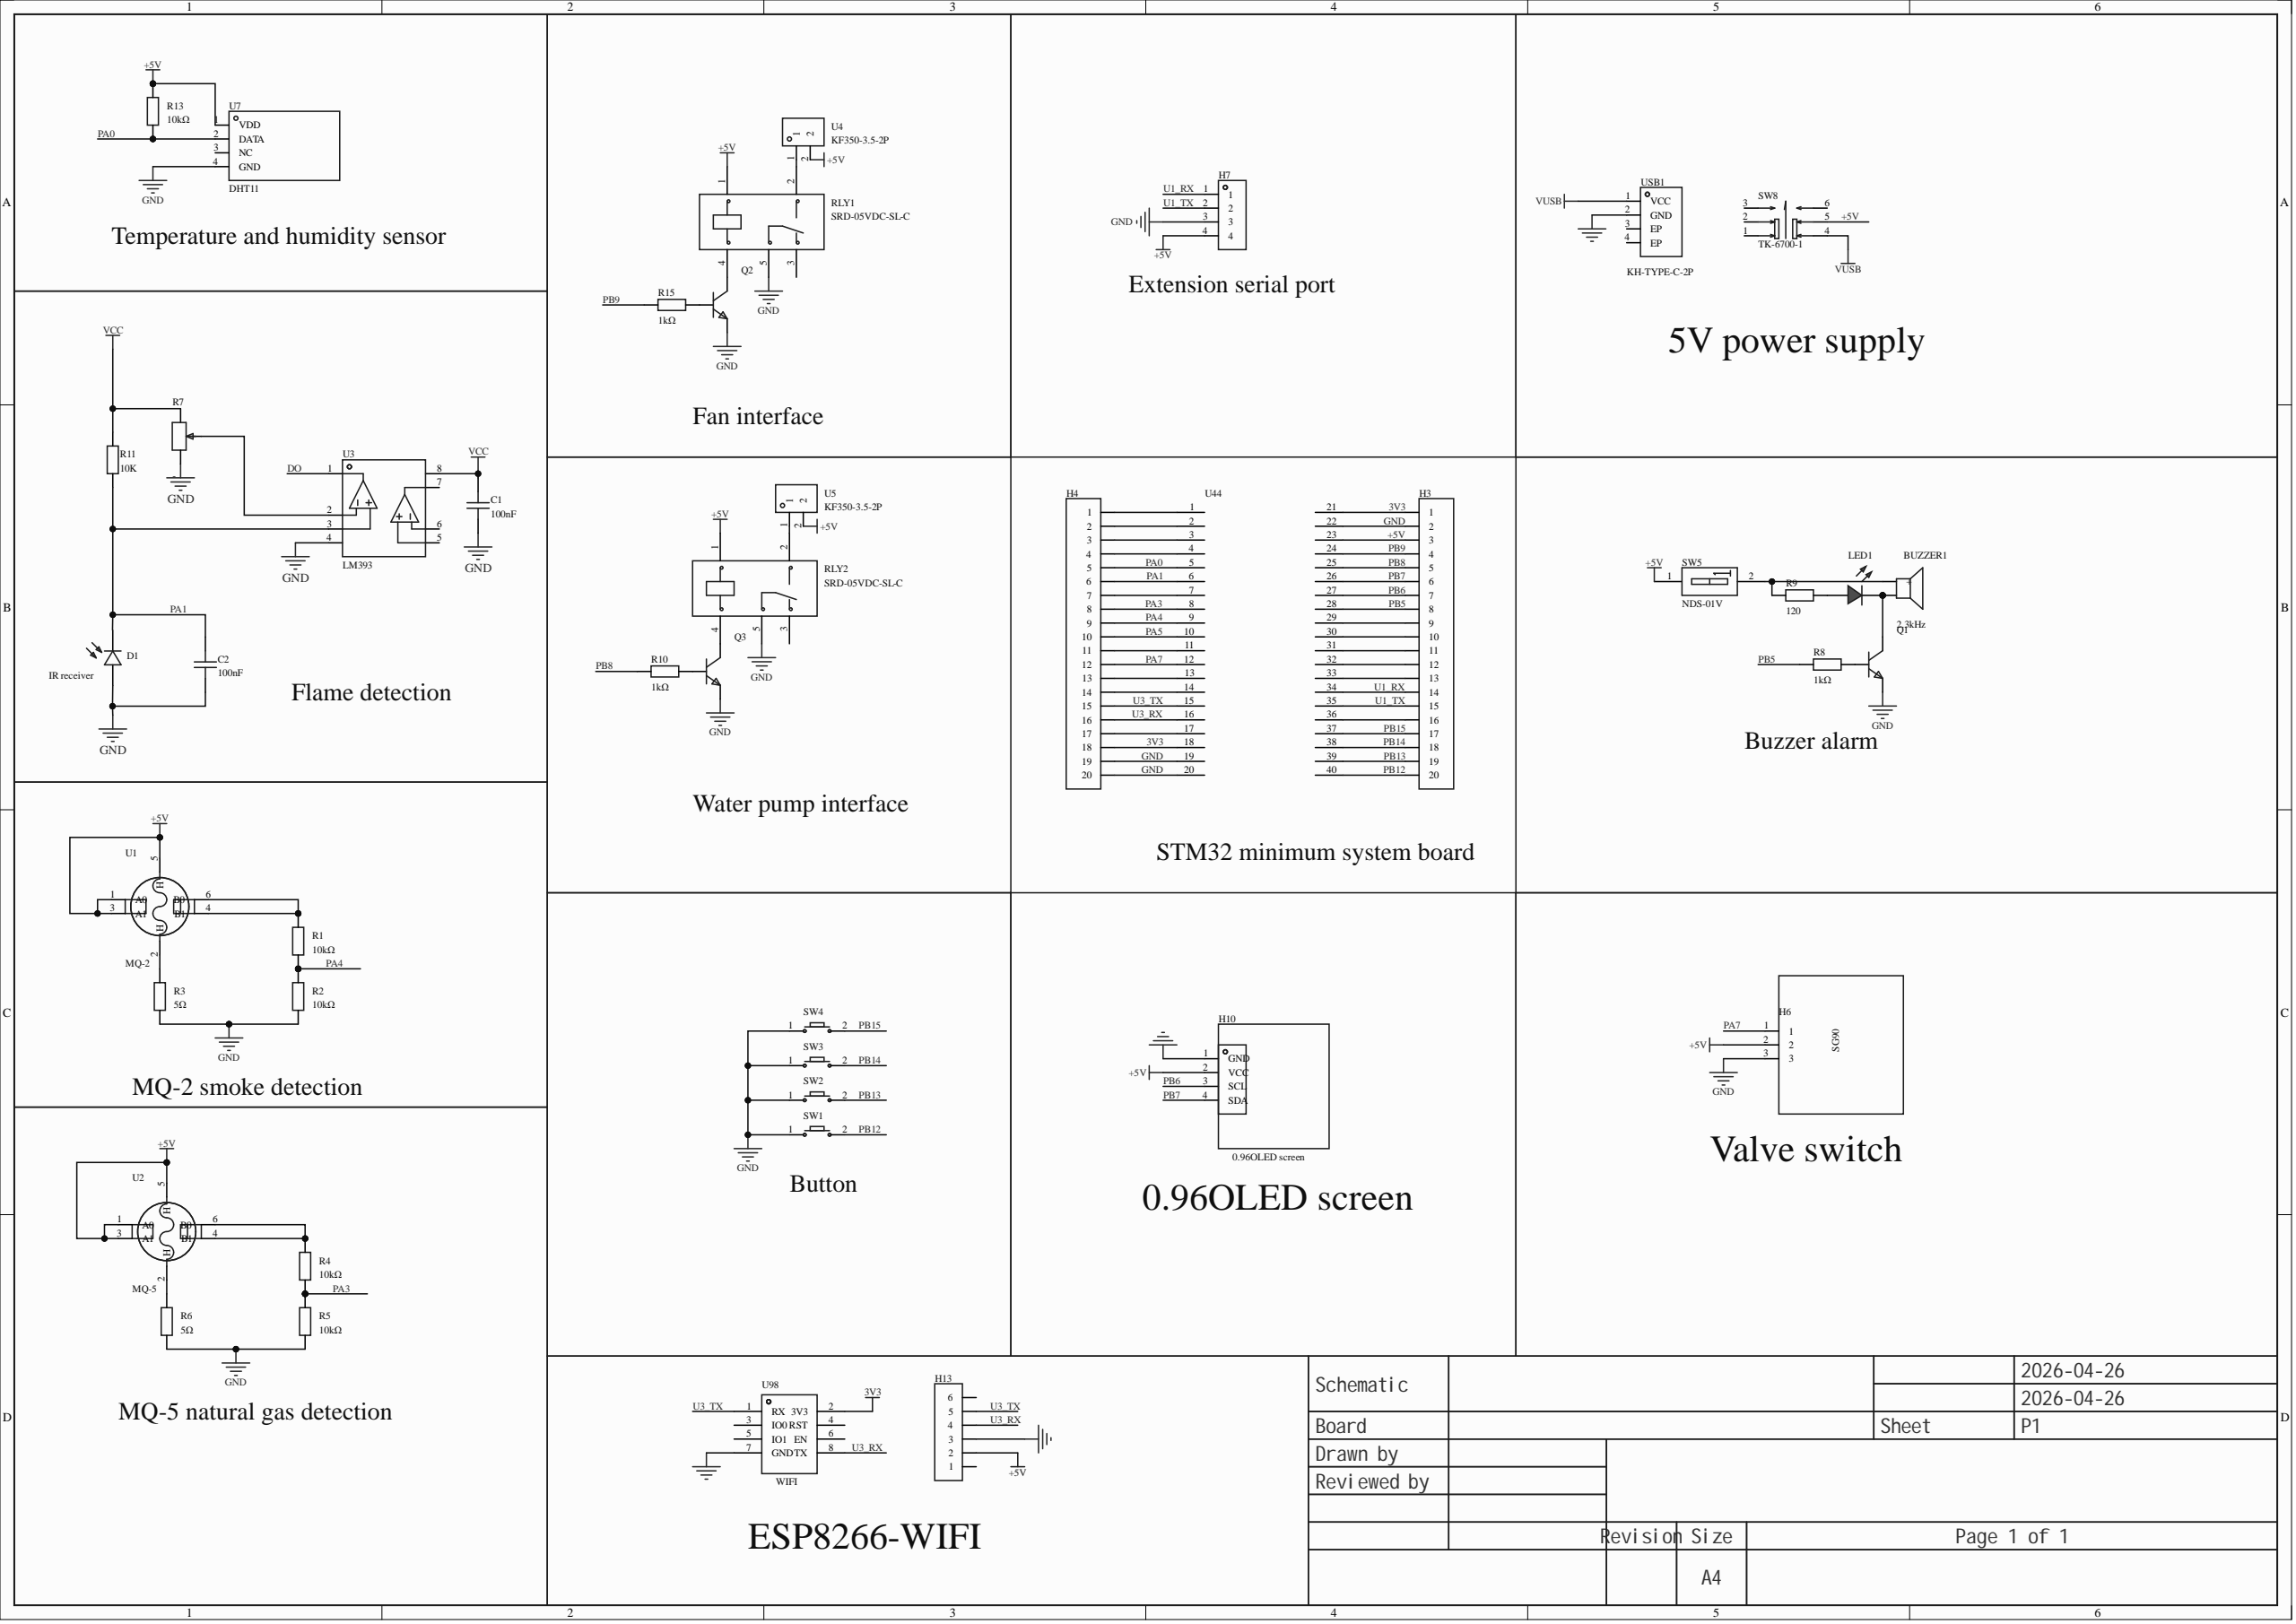Circuit board | Altium Designer | 44 parts | 54 nets
Bill of materials:
Comment,Description,Designator,Footprint,LibRef,Quantity
"2.3kHz","Drive mode: active (built-in driver circuit); construction type: electromagnetic; rated voltage: 5V; frequency: 2.3kHz; sound pressure (SPL): 85dB@5V,10cm;","BUZZER1","BUZ-TH_BD12.0-P7.60-D0.6-FD","TMB12A05_C96093","1"
"100nF","","C1, C2","C0603","CAP_0603","2"
"IR receiver","","D1","IR 接收 D5","红外接收","1"
"","","H3, H4","HDR-TH_20P-P2.54-V-F","HDR-F_2.54_1x20P","2"
"","","H6","HDR-TH_3P-P2.54-V-F","HDR-F_2.54_1x3P","1"
"","","H7","HDR-TH_4P-P2.54-V-F","HDR-F_2.54_1x4P","1"
"2.54-1*4P female","插孔结构:1x4P;间距:2.54mm;行距:-;圆孔/方孔:方孔;安装类型:直插;排数:单排;总孔位数:4P;额定电流:3A;额定电压:-;插孔方向:顶部;塑高:-;触头材质:青铜;触头镀层:-;工作温度范围:-40℃~+105℃;焊接温度(最大值):-;","H10","HDR-TH_4P-P2.54-V-F","0.96OLED屏幕","1"
"","","H13","HDR-TH_6P-P2.54-V-M-1","HDR-M_2.54_1x6P","1"
"","","LED1","LED_TH-3mm","LED_TH-R_3mm","1"
"","","Q1, Q2, Q3","S8050_TO_92","S8050_TO_NPN","3"
"10kΩ","","R1, R2, R4, R5, R13","Res_1/4W","Res_AXIAL-1/8W","5"
"5Ω","","R3, R6","Res_1/4W","Res_AXIAL-1/8W","2"
"-","Resistance: -; power: -;","R7","RES-ADJ-TH_3362P","3362P-1-103_C5047","1"
"1kΩ","","R8, R10, R15","Res_1/4W","Res_AXIAL-1/4W, Res_AXIAL-1/8W","3"
"120","","R9","Res_1/4W","Res_AXIAL-1/4W","1"
"10K","","R11","R0805","Res_0805","1"
"SRD-05VDC-SL-C","Coil voltage: 5V; contact form: one changeover: 1C (SPDT); contact rating (resistive load): -; max switching voltage: 250V@AC; max switching current: 15A;","RLY1, RLY2","RELAY-TH_SRD-XXVDC-XL-C","SRD-05VDC-SL-C","2"
"","","SW1, SW2, SW3, SW4","Key_SMD_3x4x2","Key_SMD_3x4x2","4"
"NDS-01V","Forward-toggle high lever","SW5","SW-TH_2P-L3.9-W9.9-P2.54-LS7.6","NDS-01V_C501305","1"
"TK-6700-1","","SW8","SW-TH_TK-6700-1","TK-6700-1","1"
"MQ-2","","U1","SENSOR-TH_MQ-2","MQ-2","1"
"MQ-5","","U2","SENSOR-TH_MQ-2","MQ-2","1"
"LM393","","U3","SOP-8_L4.9-W3.9-P1.27-LS6.0-BL","LM393","1"
"KF350-3.5-2P","结构:1x2P;间距:3.5mm;颜色:绿色;安装方式:直插;额定电流:10A;额定电压:300V;排数:1;线规 - AWG:18~24;线规 - 平方毫米:0.75;每排PIN数:2;工作温度范围:-40℃~+105℃;","U4, U5","CONN-TH_P3.50_KF350-3.5-2P","KF350-3.5-2P","2"
"DHT11","Temperature range: -20℃~+60℃; humidity range: 5%RH~95%RH; humidity accuracy: ±5%RH;","U7","SENSOR-TH_DHT11","DHT11","1"
"","","U44","STM32最小系统板","STM32最小系统板","1"
"","","U98","WiFi封装","WiFi模块","1"
"KH-TYPE-C-2P","Connector type: Type-C; standard: -; male/female: -; number of ports: -; number of contacts: 2P; mounting: -; rated current - power: -; contact material: -; contact plating: -; operating temperature range: -;","USB1","USB-SMD_KH-TYPE-C-2P","KH-TYPE-C-2P","1"
Netlist (Protel format):
[
BUZZER1
BUZ-TH_BD12.0-P7.60-D0.6-FD
2.3kHz



]
[
C1
C0603
100nF



]
[
C2
C0603
100nF



]
[
D1
IR 接收 D5
IR receiver



]
[
H3
HDR-TH_20P-P2.54-V-F




]
[
H4
HDR-TH_20P-P2.54-V-F




]
[
H6
HDR-TH_3P-P2.54-V-F




]
[
H7
HDR-TH_4P-P2.54-V-F




]
[
H10
HDR-TH_4P-P2.54-V-F
2.54-1*4P female



]
[
H13
HDR-TH_6P-P2.54-V-M-1




]
[
LED1
LED_TH-3mm




]
[
Q1
S8050_TO_92




]
[
Q2
S8050_TO_92




]
[
Q3
S8050_TO_92




]
[
R1
Res_1/4W
10kΩ



]
[
R2
Res_1/4W
10kΩ



]
[
R3
Res_1/4W
5Ω



]
[
R4
Res_1/4W
10kΩ



]
[
R5
Res_1/4W
10kΩ



]
[
R6
Res_1/4W
5Ω



]
[
R7
RES-ADJ-TH_3362P
-



]
[
R8
Res_1/4W
1kΩ



]
[
R9
Res_1/4W
120



]
[
R10
Res_1/4W
1kΩ



]
[
R11
R0805
10K



]
[
R13
Res_1/4W
10kΩ



]
[
R15
Res_1/4W
1kΩ



]
[
RLY1
RELAY-TH_SRD-XXVDC-XL-C
SRD-05VDC-SL-C



]
[
RLY2
RELAY-TH_SRD-XXVDC-XL-C
SRD-05VDC-SL-C



]
[
SW1
Key_SMD_3x4x2




]
[
SW2
Key_SMD_3x4x2




]
[
SW3
Key_SMD_3x4x2




]
[
SW4
Key_SMD_3x4x2




]
[
SW5
SW-TH_2P-L3.9-W9.9-P2.54-LS7.6
NDS-01V



]
[
SW8
SW-TH_TK-6700-1
TK-6700-1



]
[
U1
SENSOR-TH_MQ-2
MQ-2



]
[
U2
SENSOR-TH_MQ-2
MQ-5



]
[
U3
SOP-8_L4.9-W3.9-P1.27-LS6.0-BL
LM393



]
[
U4
CONN-TH_P3.50_KF350-3.5-2P
KF350-3.5-2P



]
[
U5
CONN-TH_P3.50_KF350-3.5-2P
KF350-3.5-2P



]
[
U7
SENSOR-TH_DHT11
DHT11



]
[
U44
STM32最小系统板




]
[
U98
WiFi封装




]
[
USB1
USB-SMD_KH-TYPE-C-2P
KH-TYPE-C-2P



]
(
VUSB
SW8-4
USB1-1
)
(
VCC
C1-2
R7-1
R11-2
U3-8
)
(
U3_TX
H4-15
H13-5
U44-15
U98-1
)
(
U3_RX
H4-16
H13-4
U44-16
U98-8
)
(
U1_TX
H3-15
H7-2
U44-35
)
(
U1_RX
H3-14
H7-1
U44-34
)
(
PB15
H3-17
SW4-2
U44-37
)
(
PB14
H3-18
SW3-2
U44-38
)
(
PB13
H3-19
SW2-2
U44-39
)
(
PB12
H3-20
SW1-2
U44-40
)
(
PB9
H3-4
R15-1
U44-24
)
(
PB8
H3-5
R10-1
U44-25
)
(
PB7
H3-6
H10-4
U44-26
)
(
PB6
H3-7
H10-3
U44-27
)
(
PB5
H3-8
R8-1
U44-28
)
(
PA7
H4-12
H6-1
U44-12
)
(
PA5
H4-10
U44-10
)
(
PA4
H4-9
R1-1
R2-2
U44-9
)
(
PA3
H4-8
R4-1
R5-2
U44-8
)
(
PA1
C2-2
H4-6
R11-1
U3-3
U44-6
)
(
PA0
H4-5
R13-1
U7-2
U44-5
)
(
NetRLY2_2
RLY2-2
U5-1
)
(
NetRLY1_2
RLY1-2
U4-1
)
(
NetR7_2
R7-2
U3-2
)
(
NetR6_2
R6-2
U2-2
)
(
NetR4_2
R4-2
U2-4
U2-6
)
(
NetR3_2
R3-2
U1-2
)
(
NetR1_2
R1-2
U1-4
U1-6
)
(
NetQ3_3
Q3-3
RLY2-4
)
(
NetQ3_2
Q3-2
R10-2
)
(
NetQ2_3
Q2-3
RLY1-4
)
(
NetQ2_2
Q2-2
R15-2
)
(
NetQ1_2
Q1-2
R8-2
)
(
NetLED1_1
LED1-1
R9-2
)
(
NetH4_17
H4-17
U44-17
)
(
NetH4_14
H4-14
U44-14
)
(
NetH4_13
H4-13
U44-13
)
(
NetH4_11
H4-11
U44-11
)
(
NetH4_7
H4-7
U44-7
)
(
NetH4_4
H4-4
U44-4
)
(
NetH4_3
H4-3
U44-3
)
(
NetH4_2
H4-2
U44-2
)
(
NetH4_1
H4-1
U44-1
)
(
NetH3_16
H3-16
U44-36
)
(
NetH3_13
H3-13
U44-33
)
(
NetH3_12
H3-12
U44-32
)
(
NetH3_11
H3-11
U44-31
)
(
NetH3_10
H3-10
U44-30
)
(
NetH3_9
H3-9
U44-29
)
(
NetBUZZER1_2
BUZZER1-2
LED1-2
Q1-3
)
(
NetBUZZER1_1
BUZZER1-1
R9-1
SW5-2
)
(
GND
C1-1
C2-1
D1-1
H3-2
H4-19
H4-20
H6-3
H7-3
H10-1
H13-3
Q1-1
Q2-1
Q3-1
R2-1
R3-1
R5-1
R6-1
R7-3
RLY1-5
RLY2-5
SW1-1
SW2-1
SW3-1
SW4-1
U3-4
U7-4
U44-19
U44-20
U44-22
U98-7
USB1-2
)
(
+5V
H3-3
H6-2
H7-4
H10-2
H13-2
R13-2
RLY1-1
RLY2-1
SW5-1
SW8-5
U1-1
U1-3
U1-5
U2-1
U2-3
U2-5
U4-2
U5-2
U7-1
U44-23
)
(
3V3
H3-1
H4-18
U44-18
U44-21
U98-2
)